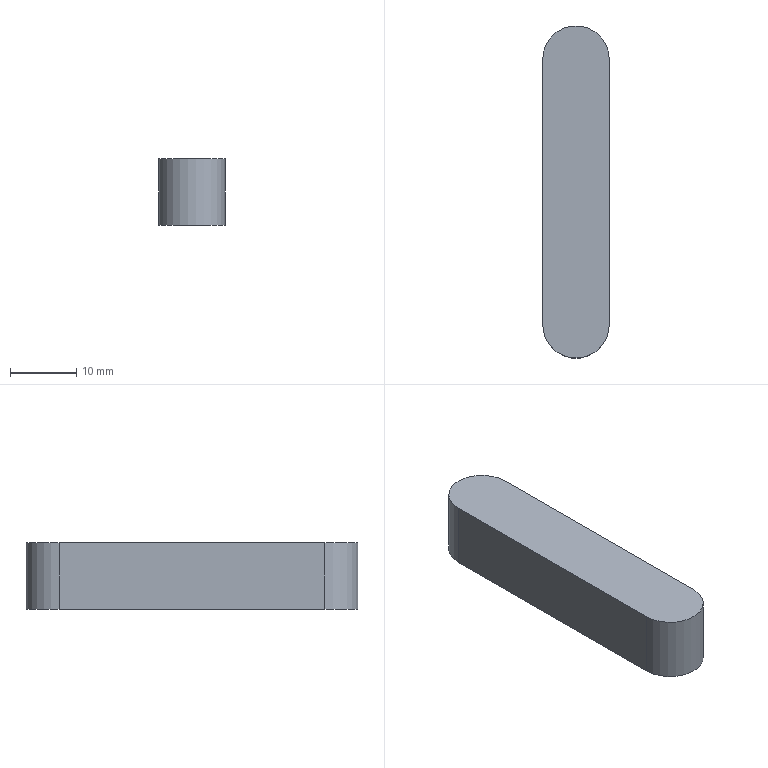Part | NX | features DATUM_CSYS 2, BLEND 1, EXTRUDE 1, SKETCH 1 | 1 solid | 6 faces | box 10 x 50 x 10 mm | volume 4785 mm3 | plane 4 | cylinder 2 | commonest cylinder face diameters 10 x2
STEP:
#1=CARTESIAN_POINT('',(-5.,20.,10.));
#2=VERTEX_POINT('',#1);
#3=CARTESIAN_POINT('',(-5.,-20.,10.));
#4=VERTEX_POINT('',#3);
#5=CARTESIAN_POINT('',(-5.,25.,10.));
#6=DIRECTION('',(0.,-1.,0.));
#7=VECTOR('',#6,1000.);
#8=LINE('',#5,#7);
#9=EDGE_CURVE('',#2,#4,#8,.T.);
#10=ORIENTED_EDGE('',*,*,#9,.F.);
#11=CARTESIAN_POINT('',(-5.,20.,0.));
#12=VERTEX_POINT('',#11);
#13=CARTESIAN_POINT('',(-5.,20.,10.));
#14=DIRECTION('',(0.,0.,-1.));
#15=VECTOR('',#14,1000.);
#16=LINE('',#13,#15);
#17=EDGE_CURVE('',#2,#12,#16,.T.);
#18=ORIENTED_EDGE('',*,*,#17,.T.);
#19=CARTESIAN_POINT('',(-5.,-20.,0.));
#20=VERTEX_POINT('',#19);
#21=CARTESIAN_POINT('',(-5.,25.,0.));
#22=DIRECTION('',(0.,-1.,0.));
#23=VECTOR('',#22,1000.);
#24=LINE('',#21,#23);
#25=EDGE_CURVE('',#12,#20,#24,.T.);
#26=ORIENTED_EDGE('',*,*,#25,.T.);
#27=CARTESIAN_POINT('',(-5.,-20.,10.));
#28=DIRECTION('',(0.,0.,-1.));
#29=VECTOR('',#28,1000.);
#30=LINE('',#27,#29);
#31=EDGE_CURVE('',#20,#4,#30,.F.);
#32=ORIENTED_EDGE('',*,*,#31,.T.);
#33=EDGE_LOOP('',(#10,#18,#26,#32));
#34=FACE_BOUND('',#33,.T.);
#35=CARTESIAN_POINT('',(-5.,25.,10.));
#36=DIRECTION('',(1.,0.,0.));
#37=DIRECTION('',(0.,0.,-1.));
#38=AXIS2_PLACEMENT_3D('',#35,#36,#37);
#39=PLANE('',#38);
#40=ADVANCED_FACE('',(#34),#39,.F.);
#41=CARTESIAN_POINT('',(5.,-20.,0.));
#42=VERTEX_POINT('',#41);
#43=CARTESIAN_POINT('',(5.,20.,0.));
#44=VERTEX_POINT('',#43);
#45=CARTESIAN_POINT('',(5.,-25.,0.));
#46=DIRECTION('',(0.,1.,0.));
#47=VECTOR('',#46,1000.);
#48=LINE('',#45,#47);
#49=EDGE_CURVE('',#42,#44,#48,.T.);
#50=ORIENTED_EDGE('',*,*,#49,.T.);
#51=CARTESIAN_POINT('',(5.,20.,10.));
#52=VERTEX_POINT('',#51);
#53=CARTESIAN_POINT('',(5.,20.,10.));
#54=DIRECTION('',(0.,0.,-1.));
#55=VECTOR('',#54,1000.);
#56=LINE('',#53,#55);
#57=EDGE_CURVE('',#44,#52,#56,.F.);
#58=ORIENTED_EDGE('',*,*,#57,.T.);
#59=CARTESIAN_POINT('',(5.,-20.,10.));
#60=VERTEX_POINT('',#59);
#61=CARTESIAN_POINT('',(5.,-25.,10.));
#62=DIRECTION('',(0.,1.,0.));
#63=VECTOR('',#62,1000.);
#64=LINE('',#61,#63);
#65=EDGE_CURVE('',#60,#52,#64,.T.);
#66=ORIENTED_EDGE('',*,*,#65,.F.);
#67=CARTESIAN_POINT('',(5.,-20.,10.));
#68=DIRECTION('',(0.,0.,-1.));
#69=VECTOR('',#68,1000.);
#70=LINE('',#67,#69);
#71=EDGE_CURVE('',#60,#42,#70,.T.);
#72=ORIENTED_EDGE('',*,*,#71,.T.);
#73=EDGE_LOOP('',(#50,#58,#66,#72));
#74=FACE_BOUND('',#73,.T.);
#75=CARTESIAN_POINT('',(5.,-25.,10.));
#76=DIRECTION('',(-1.,0.,0.));
#77=DIRECTION('',(0.,0.,1.));
#78=AXIS2_PLACEMENT_3D('',#75,#76,#77);
#79=PLANE('',#78);
#80=ADVANCED_FACE('',(#74),#79,.F.);
#81=CARTESIAN_POINT('',(0.,20.,10.));
#82=DIRECTION('',(0.,0.,1.));
#83=DIRECTION('',(1.,0.,0.));
#84=AXIS2_PLACEMENT_3D('',#81,#82,#83);
#85=CIRCLE('',#84,5.);
#86=EDGE_CURVE('',#52,#2,#85,.T.);
#87=ORIENTED_EDGE('',*,*,#86,.T.);
#88=ORIENTED_EDGE('',*,*,#9,.T.);
#89=CARTESIAN_POINT('',(0.,-20.,10.));
#90=DIRECTION('',(0.,0.,1.));
#91=DIRECTION('',(1.,0.,0.));
#92=AXIS2_PLACEMENT_3D('',#89,#90,#91);
#93=CIRCLE('',#92,5.);
#94=EDGE_CURVE('',#4,#60,#93,.T.);
#95=ORIENTED_EDGE('',*,*,#94,.T.);
#96=ORIENTED_EDGE('',*,*,#65,.T.);
#97=EDGE_LOOP('',(#87,#88,#95,#96));
#98=FACE_BOUND('',#97,.T.);
#99=CARTESIAN_POINT('',(0.,0.,10.));
#100=DIRECTION('',(0.,0.,1.));
#101=DIRECTION('',(1.,0.,0.));
#102=AXIS2_PLACEMENT_3D('',#99,#100,#101);
#103=PLANE('',#102);
#104=ADVANCED_FACE('',(#98),#103,.T.);
#105=ORIENTED_EDGE('',*,*,#25,.F.);
#106=CARTESIAN_POINT('',(0.,20.,0.));
#107=DIRECTION('',(0.,0.,1.));
#108=DIRECTION('',(1.,0.,0.));
#109=AXIS2_PLACEMENT_3D('',#106,#107,#108);
#110=CIRCLE('',#109,5.);
#111=EDGE_CURVE('',#12,#44,#110,.F.);
#112=ORIENTED_EDGE('',*,*,#111,.T.);
#113=ORIENTED_EDGE('',*,*,#49,.F.);
#114=CARTESIAN_POINT('',(0.,-20.,0.));
#115=DIRECTION('',(0.,0.,1.));
#116=DIRECTION('',(1.,0.,0.));
#117=AXIS2_PLACEMENT_3D('',#114,#115,#116);
#118=CIRCLE('',#117,5.);
#119=EDGE_CURVE('',#42,#20,#118,.F.);
#120=ORIENTED_EDGE('',*,*,#119,.T.);
#121=EDGE_LOOP('',(#105,#112,#113,#120));
#122=FACE_BOUND('',#121,.T.);
#123=CARTESIAN_POINT('',(0.,0.,0.));
#124=DIRECTION('',(0.,0.,1.));
#125=DIRECTION('',(1.,0.,0.));
#126=AXIS2_PLACEMENT_3D('',#123,#124,#125);
#127=PLANE('',#126);
#128=ADVANCED_FACE('',(#122),#127,.F.);
#129=ORIENTED_EDGE('',*,*,#111,.F.);
#130=ORIENTED_EDGE('',*,*,#17,.F.);
#131=ORIENTED_EDGE('',*,*,#86,.F.);
#132=ORIENTED_EDGE('',*,*,#57,.F.);
#133=EDGE_LOOP('',(#129,#130,#131,#132));
#134=FACE_BOUND('',#133,.T.);
#135=CARTESIAN_POINT('',(0.,20.,10.));
#136=DIRECTION('',(0.,0.,-1.));
#137=DIRECTION('',(-1.,0.,0.));
#138=AXIS2_PLACEMENT_3D('',#135,#136,#137);
#139=CYLINDRICAL_SURFACE('',#138,5.);
#140=ADVANCED_FACE('',(#134),#139,.T.);
#141=ORIENTED_EDGE('',*,*,#71,.F.);
#142=ORIENTED_EDGE('',*,*,#94,.F.);
#143=ORIENTED_EDGE('',*,*,#31,.F.);
#144=ORIENTED_EDGE('',*,*,#119,.F.);
#145=EDGE_LOOP('',(#141,#142,#143,#144));
#146=FACE_BOUND('',#145,.T.);
#147=CARTESIAN_POINT('',(0.,-20.,10.));
#148=DIRECTION('',(0.,0.,-1.));
#149=DIRECTION('',(-1.,0.,0.));
#150=AXIS2_PLACEMENT_3D('',#147,#148,#149);
#151=CYLINDRICAL_SURFACE('',#150,5.);
#152=ADVANCED_FACE('',(#146),#151,.T.);
#153=CLOSED_SHELL('',(#40,#80,#104,#128,#140,#152));
#154=MANIFOLD_SOLID_BREP('',#153);
#155=(LENGTH_UNIT()NAMED_UNIT(*)SI_UNIT(.MILLI.,.METRE.));
#156=UNCERTAINTY_MEASURE_WITH_UNIT(LENGTH_MEASURE(0.00001),#155,'','');
#157=(NAMED_UNIT(*)PLANE_ANGLE_UNIT()SI_UNIT($,.RADIAN.));
#158=(NAMED_UNIT(*)SI_UNIT($,.STERADIAN.)SOLID_ANGLE_UNIT());
#159=(GEOMETRIC_REPRESENTATION_CONTEXT(3)GLOBAL_UNCERTAINTY_ASSIGNED_CONTEXT((#156))GLOBAL_UNIT_ASSIGNED_CONTEXT((#155,#157,#158))REPRESENTATION_CONTEXT('',''));
#160=ADVANCED_BREP_SHAPE_REPRESENTATION('',(#154),#159);